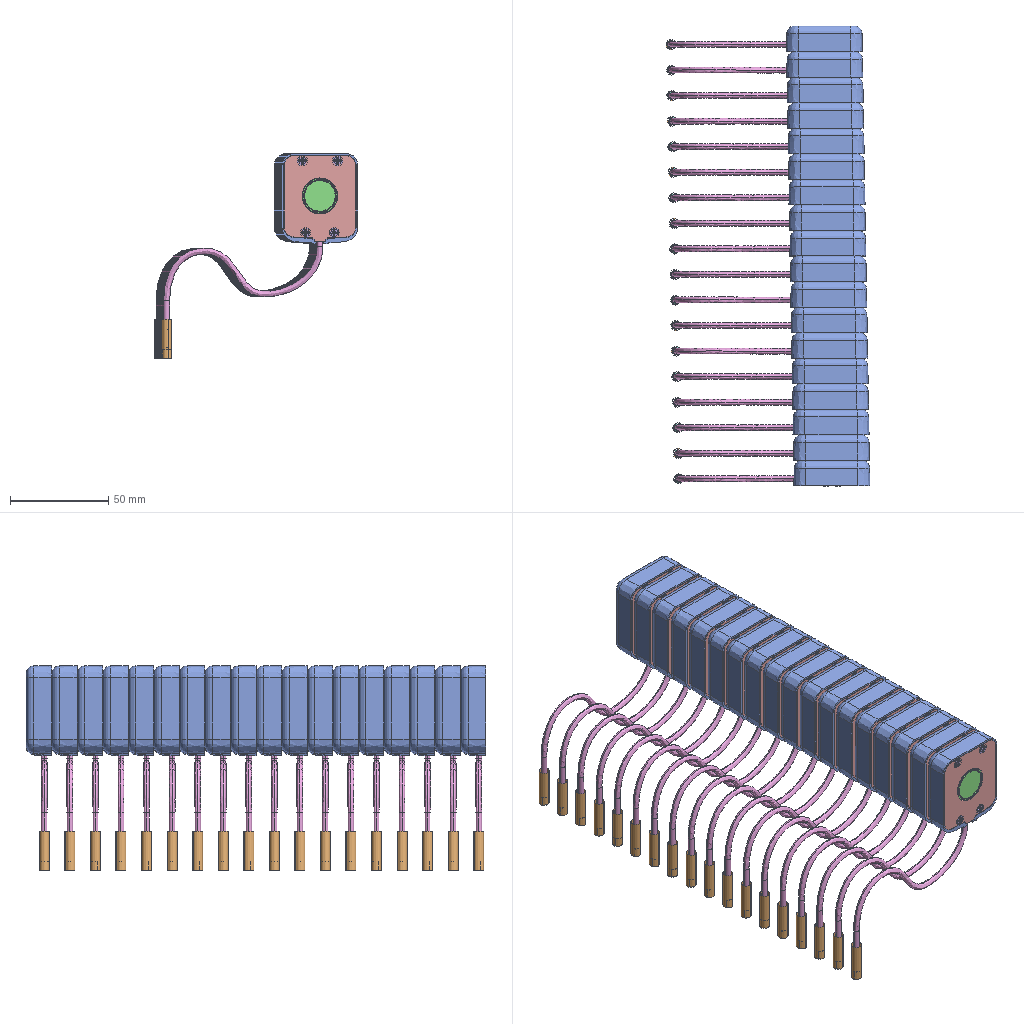Assembly | SolidWorks | 8 different items | 198 placed | box 104 x 234 x 104 mm
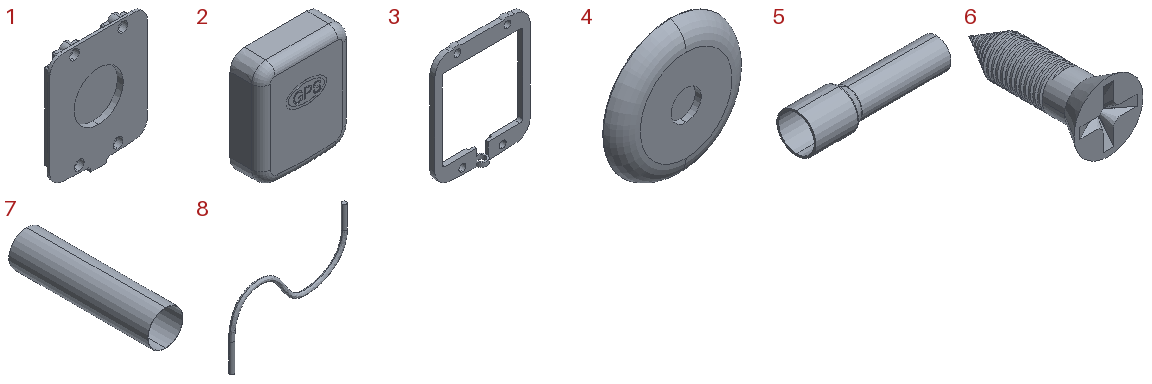Parts list (item | quantity | size | volume | features):
1 | x18 | 36.5 x 3.7 x 43.598 mm | 2859 mm3 | features ICE 7, Extrusion 1, RevCut 1
2 | x18 | 38.7 x 13 x 46 mm | 6467 mm3 | features ICE 11, Fillet 4, Extrusion 1, RevCut 1
3 | x18 | 34.4 x 4.123 x 41.42 mm | 850.585 mm3 | features ICE 5, Extrusion 1
4 | x18 | 17.931 x 2.2 x 17.931 mm | 454.739 mm3 | features Revolution 1
5 | x18 | 15 x 4.2 x 4.2 mm | 31.684 mm3 | features Revolution 1
6 | x72 | 5.2 x 10.5 x 5.2 mm | 67.225 mm3 | features BlendCut 1, Helix 1, ICE 1, Revolution 1, SweepCut 1
7 | x18 | 5.1 x 20 x 5.1 mm | 15.865 mm3 | features ExtruThin 1
8 | x18 | 81 x 3 x 63.219 mm | 1077 mm3 | features Sweep 1
Mates (type | each side: item.copy, entity, surface, feature):
Coordinate | 1.1 select_type:25 | assembly select_type:11
Coincident | 1.1 face cylinder Boss-Extrude6 | 2.1 select_type:24
Coincident | 2.1 plane | assembly plane
Coincident | 1.1 face plane Boss-Extrude1 | 2.1 face plane Boss-Extrude 1
Coincident | 2.1 plane | 3.1 plane
Coincident | 2.1 face plane Boss-Extrude2 | 3.1 face plane Boss-Extrude 1
DistanceDim | 3.1 plane | 2.1 plane
Concentric | 1.1 face cylinder Cut-Revolve1 | 8.1 face cylinder Sweep1
Parallel | 8.1 plane | assembly plane
Concentric | 5.1 face cylinder Revolve 1 | 7.1 face cylinder Extrude-Thin1
Concentric | 1.1 face cylinder Cut-Extrude2 | 6.1 edge
DistanceDim | 1.1 face plane Boss-Extrude1 | 6.1 face plane Revolve2
Concentric | 1.1 face cylinder Cut-Extrude1 | 6.2 edge
DistanceDim | 1.1 face plane Boss-Extrude1 | 6.2 face plane Revolve2
Concentric | 1.1 face cylinder Cut-Extrude2 | 6.3 edge
DistanceDim | 1.1 face plane Boss-Extrude1 | 6.3 face plane Revolve2
Concentric | 1.1 face cylinder Cut-Extrude2 | 6.4 edge
DistanceDim | 1.1 face plane Boss-Extrude1 | 6.4 face plane Revolve2
Concentric | 1.1 edge | 4.1 edge
Coincident | 1.1 face plane Cut-Extrude2 | 4.1 face plane Revolve1